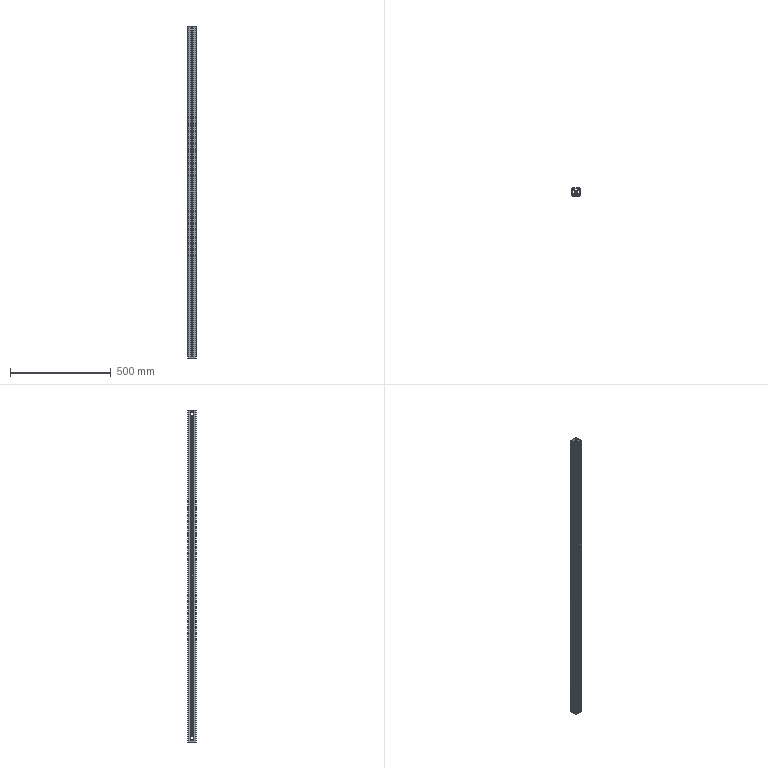Part | SolidWorks | features BaseBody 1, HoleWzd 1, MoveFace 1 | 1 solid | 242 faces | box 40 x 40 x 1650 mm | volume 968537 mm3 | plane 187 | cylinder 55 | commonest cylinder face diameters 6.8 x15 2 x14 19 x12 1 x6 5 x4 9 x4